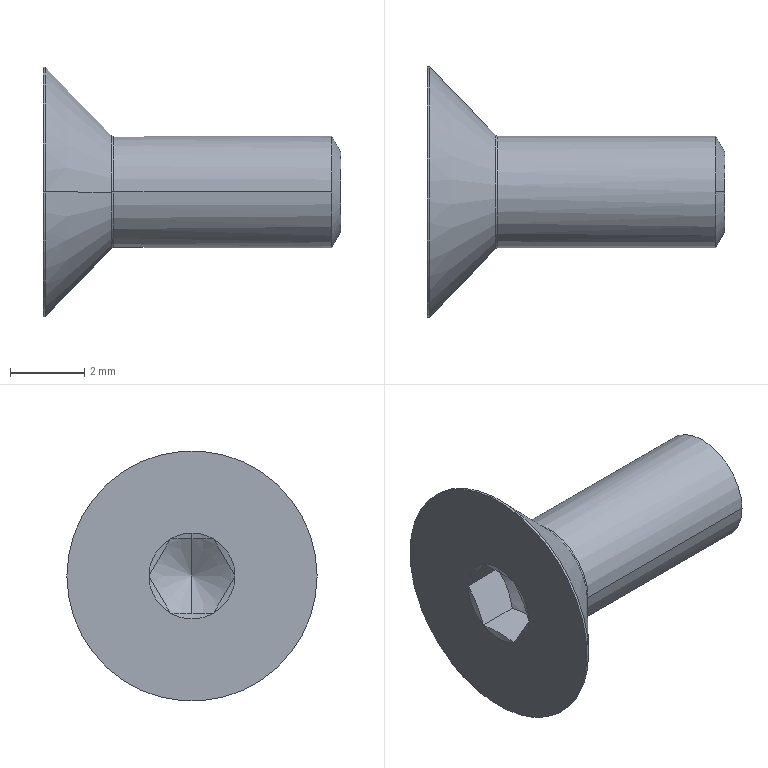Part | SolidWorks | features RevCut 2, Revolution 2, Cut 1, LPattern 1, RefAxis 1 | 1 solid | 27 faces | box 8 x 6.72 x 6.72 mm | volume 75.425 mm3 | cone 13 | plane 8 | cylinder 4 | torus 2 | commonest cylinder face diameters 3 x2 6.72 x2
STEP:
#1=CARTESIAN_POINT('',(0.,0.,1.067));
#2=VERTEX_POINT('',#1);
#3=CARTESIAN_POINT('',(0.,0.,-1.067));
#4=VERTEX_POINT('',#3);
#5=CARTESIAN_POINT('',(0.,0.,0.));
#6=DIRECTION('',(-1.,0.,0.));
#7=DIRECTION('',(0.,0.,1.));
#8=AXIS2_PLACEMENT_3D('',#5,#6,#7);
#9=CIRCLE('',#8,1.067);
#10=EDGE_CURVE('',#2,#4,#9,.T.);
#11=ORIENTED_EDGE('',*,*,#10,.T.);
#12=CARTESIAN_POINT('',(-0.25,0.,-1.5));
#13=VERTEX_POINT('',#12);
#14=CARTESIAN_POINT('',(-0.25,0.,-1.5));
#15=DIRECTION('',(-0.5,0.,-0.866));
#16=VECTOR('',#15,1000.);
#17=LINE('',#14,#16);
#18=EDGE_CURVE('',#4,#13,#17,.T.);
#19=ORIENTED_EDGE('',*,*,#18,.T.);
#20=CARTESIAN_POINT('',(-0.25,1.5,0.));
#21=VERTEX_POINT('',#20);
#22=CARTESIAN_POINT('',(-0.25,0.,0.));
#23=DIRECTION('',(-1.,0.,0.));
#24=DIRECTION('',(0.,0.,1.));
#25=AXIS2_PLACEMENT_3D('',#22,#23,#24);
#26=CIRCLE('',#25,1.5);
#27=EDGE_CURVE('',#21,#13,#26,.T.);
#28=ORIENTED_EDGE('',*,*,#27,.F.);
#29=CARTESIAN_POINT('',(-0.25,0.,1.5));
#30=VERTEX_POINT('',#29);
#31=CARTESIAN_POINT('',(-0.25,0.,0.));
#32=DIRECTION('',(-1.,0.,0.));
#33=DIRECTION('',(0.,0.,1.));
#34=AXIS2_PLACEMENT_3D('',#31,#32,#33);
#35=CIRCLE('',#34,1.5);
#36=EDGE_CURVE('',#30,#21,#35,.T.);
#37=ORIENTED_EDGE('',*,*,#36,.F.);
#38=CARTESIAN_POINT('',(-0.25,0.,1.5));
#39=DIRECTION('',(-0.5,0.,0.866));
#40=VECTOR('',#39,1000.);
#41=LINE('',#38,#40);
#42=EDGE_CURVE('',#2,#30,#41,.T.);
#43=ORIENTED_EDGE('',*,*,#42,.F.);
#44=EDGE_LOOP('',(#11,#19,#28,#37,#43));
#45=FACE_OUTER_BOUND('',#44,.T.);
#46=CARTESIAN_POINT('',(-0.25,0.,0.));
#47=DIRECTION('',(-1.,0.,0.));
#48=DIRECTION('',(0.,0.,1.));
#49=AXIS2_PLACEMENT_3D('',#46,#47,#48);
#50=CONICAL_SURFACE('',#49,1.5,1.047);
#51=ADVANCED_FACE('',(#45),#50,.T.);
#52=CARTESIAN_POINT('',(-6.233,0.,0.));
#53=VERTEX_POINT('',#52);
#54=CARTESIAN_POINT('',(-6.811,0.,1.));
#55=VERTEX_POINT('',#54);
#56=CARTESIAN_POINT('',(-6.9,0.,1.155));
#57=DIRECTION('',(-0.5,0.,0.866));
#58=VECTOR('',#57,1000.);
#59=LINE('',#56,#58);
#60=EDGE_CURVE('',#53,#55,#59,.T.);
#61=ORIENTED_EDGE('',*,*,#60,.F.);
#62=CARTESIAN_POINT('',(-6.811,0.,-1.));
#63=VERTEX_POINT('',#62);
#64=CARTESIAN_POINT('',(-6.9,0.,-1.155));
#65=DIRECTION('',(-0.5,0.,-0.866));
#66=VECTOR('',#65,1000.);
#67=LINE('',#64,#66);
#68=EDGE_CURVE('',#53,#63,#67,.T.);
#69=ORIENTED_EDGE('',*,*,#68,.T.);
#70=CARTESIAN_POINT('',(-6.9,-0.5774,-1.));
#71=VERTEX_POINT('',#70);
#72=CARTESIAN_POINT('',(-6.811,0.,-1.));
#73=CARTESIAN_POINT('',(-6.811,-0.1949,-1.));
#74=CARTESIAN_POINT('',(-6.846,-0.3898,-1.));
#75=CARTESIAN_POINT('',(-6.9,-0.5774,-1.));
#76=B_SPLINE_CURVE_WITH_KNOTS('',3,(#72,#73,#74,#75),.UNSPECIFIED.,.F.,.F.,(4,4),(0.003677,0.004261),.UNSPECIFIED.);
#77=EDGE_CURVE('',#63,#71,#76,.T.);
#78=ORIENTED_EDGE('',*,*,#77,.T.);
#79=CARTESIAN_POINT('',(-6.9,-1.155,0.));
#80=VERTEX_POINT('',#79);
#81=CARTESIAN_POINT('',(-6.9,-0.5774,-1.));
#82=CARTESIAN_POINT('',(-6.846,-0.6716,-0.8367));
#83=CARTESIAN_POINT('',(-6.811,-0.7673,-0.671));
#84=CARTESIAN_POINT('',(-6.811,-0.9636,-0.3309));
#85=CARTESIAN_POINT('',(-6.846,-1.06,-0.1635));
#86=CARTESIAN_POINT('',(-6.9,-1.155,0.));
#87=B_SPLINE_CURVE_WITH_KNOTS('',3,(#81,#82,#83,#84,#85,#86),.UNSPECIFIED.,.F.,.F.,(4,2,4),(0.000000238,0.0005833,0.001166),.UNSPECIFIED.);
#88=EDGE_CURVE('',#71,#80,#87,.T.);
#89=ORIENTED_EDGE('',*,*,#88,.T.);
#90=CARTESIAN_POINT('',(-6.9,-0.5774,1.));
#91=VERTEX_POINT('',#90);
#92=CARTESIAN_POINT('',(-6.9,-1.155,0.));
#93=CARTESIAN_POINT('',(-6.846,-1.06,0.1633));
#94=CARTESIAN_POINT('',(-6.811,-0.9647,0.329));
#95=CARTESIAN_POINT('',(-6.811,-0.7684,0.6691));
#96=CARTESIAN_POINT('',(-6.846,-0.6717,0.8365));
#97=CARTESIAN_POINT('',(-6.9,-0.5774,1.));
#98=B_SPLINE_CURVE_WITH_KNOTS('',3,(#92,#93,#94,#95,#96,#97),.UNSPECIFIED.,.F.,.F.,(4,2,4),(0.000000238,0.0005833,0.001166),.UNSPECIFIED.);
#99=EDGE_CURVE('',#80,#91,#98,.T.);
#100=ORIENTED_EDGE('',*,*,#99,.T.);
#101=CARTESIAN_POINT('',(-6.9,-0.5774,1.));
#102=CARTESIAN_POINT('',(-6.846,-0.3898,1.));
#103=CARTESIAN_POINT('',(-6.811,-0.1949,1.));
#104=CARTESIAN_POINT('',(-6.811,0.,1.));
#105=B_SPLINE_CURVE_WITH_KNOTS('',3,(#101,#102,#103,#104),.UNSPECIFIED.,.F.,.F.,(4,4),(0.00099,0.001574),.UNSPECIFIED.);
#106=EDGE_CURVE('',#91,#55,#105,.T.);
#107=ORIENTED_EDGE('',*,*,#106,.T.);
#108=EDGE_LOOP('',(#61,#69,#78,#89,#100,#107));
#109=FACE_OUTER_BOUND('',#108,.T.);
#110=CARTESIAN_POINT('',(-6.9,0.,0.));
#111=DIRECTION('',(-1.,0.,0.));
#112=DIRECTION('',(0.,0.,1.));
#113=AXIS2_PLACEMENT_3D('',#110,#111,#112);
#114=CONICAL_SURFACE('',#113,1.155,1.047);
#115=ADVANCED_FACE('',(#109),#114,.F.);
#116=CARTESIAN_POINT('',(-8.,0.5774,1.));
#117=VERTEX_POINT('',#116);
#118=CARTESIAN_POINT('',(-7.956,0.,1.));
#119=VERTEX_POINT('',#118);
#120=CARTESIAN_POINT('',(-8.,0.5774,1.));
#121=CARTESIAN_POINT('',(-7.973,0.3853,1.));
#122=CARTESIAN_POINT('',(-7.956,0.193,1.));
#123=CARTESIAN_POINT('',(-7.956,0.,1.));
#124=B_SPLINE_CURVE_WITH_KNOTS('',3,(#120,#121,#122,#123),.UNSPECIFIED.,.F.,.F.,(4,4),(0.002431,0.003013),.UNSPECIFIED.);
#125=EDGE_CURVE('',#117,#119,#124,.T.);
#126=ORIENTED_EDGE('',*,*,#125,.T.);
#127=CARTESIAN_POINT('',(-8.,0.,1.155));
#128=VERTEX_POINT('',#127);
#129=CARTESIAN_POINT('',(-7.67,0.,0.));
#130=DIRECTION('',(-0.2748,0.,0.9615));
#131=VECTOR('',#130,1000.);
#132=LINE('',#129,#131);
#133=EDGE_CURVE('',#119,#128,#132,.T.);
#134=ORIENTED_EDGE('',*,*,#133,.T.);
#135=CARTESIAN_POINT('',(-8.,0.,0.));
#136=DIRECTION('',(1.,0.,0.));
#137=DIRECTION('',(0.,-1.,0.));
#138=AXIS2_PLACEMENT_3D('',#135,#136,#137);
#139=CIRCLE('',#138,1.155);
#140=EDGE_CURVE('',#117,#128,#139,.T.);
#141=ORIENTED_EDGE('',*,*,#140,.F.);
#142=EDGE_LOOP('',(#126,#134,#141));
#143=FACE_OUTER_BOUND('',#142,.T.);
#144=CARTESIAN_POINT('',(-1007.67,0.,0.));
#145=DIRECTION('',(-1.,0.,0.));
#146=DIRECTION('',(0.,0.,1.));
#147=AXIS2_PLACEMENT_3D('',#144,#145,#146);
#148=CONICAL_SURFACE('',#147,3499.093,1.292);
#149=ADVANCED_FACE('',(#143),#148,.F.);
#150=CARTESIAN_POINT('',(-6.098,-1.5,0.));
#151=VERTEX_POINT('',#150);
#152=CARTESIAN_POINT('',(-6.098,1.5,0.));
#153=VERTEX_POINT('',#152);
#154=CARTESIAN_POINT('',(-6.098,0.,0.));
#155=DIRECTION('',(1.,0.,0.));
#156=DIRECTION('',(0.,1.,0.));
#157=AXIS2_PLACEMENT_3D('',#154,#155,#156);
#158=CIRCLE('',#157,1.5);
#159=EDGE_CURVE('',#151,#153,#158,.T.);
#160=ORIENTED_EDGE('',*,*,#159,.F.);
#161=CARTESIAN_POINT('',(-6.169,-1.531,0.));
#162=VERTEX_POINT('',#161);
#163=CARTESIAN_POINT('',(-6.098,-1.6,0.));
#164=DIRECTION('',(0.,0.,1.));
#165=DIRECTION('',(0.,-1.,0.));
#166=AXIS2_PLACEMENT_3D('',#163,#164,#165);
#167=CIRCLE('',#166,0.1);
#168=EDGE_CURVE('',#151,#162,#167,.T.);
#169=ORIENTED_EDGE('',*,*,#168,.T.);
#170=CARTESIAN_POINT('',(-6.169,1.531,0.));
#171=VERTEX_POINT('',#170);
#172=CARTESIAN_POINT('',(-6.169,0.,0.));
#173=DIRECTION('',(1.,0.,0.));
#174=DIRECTION('',(0.,1.,0.));
#175=AXIS2_PLACEMENT_3D('',#172,#173,#174);
#176=CIRCLE('',#175,1.531);
#177=EDGE_CURVE('',#162,#171,#176,.T.);
#178=ORIENTED_EDGE('',*,*,#177,.T.);
#179=CARTESIAN_POINT('',(-6.098,1.6,0.));
#180=DIRECTION('',(0.,0.,-1.));
#181=DIRECTION('',(-1.,0.,0.));
#182=AXIS2_PLACEMENT_3D('',#179,#180,#181);
#183=CIRCLE('',#182,0.1);
#184=EDGE_CURVE('',#153,#171,#183,.T.);
#185=ORIENTED_EDGE('',*,*,#184,.F.);
#186=EDGE_LOOP('',(#160,#169,#178,#185));
#187=FACE_OUTER_BOUND('',#186,.T.);
#188=CARTESIAN_POINT('',(-6.098,0.,0.));
#189=DIRECTION('',(1.,0.,0.));
#190=DIRECTION('',(0.,1.,0.));
#191=AXIS2_PLACEMENT_3D('',#188,#189,#190);
#192=TOROIDAL_SURFACE('',#191,1.6,0.1);
#193=ADVANCED_FACE('',(#187),#192,.F.);
#194=CARTESIAN_POINT('',(-6.169,0.,0.));
#195=DIRECTION('',(1.,0.,0.));
#196=DIRECTION('',(0.,1.,0.));
#197=AXIS2_PLACEMENT_3D('',#194,#195,#196);
#198=CIRCLE('',#197,1.531);
#199=EDGE_CURVE('',#171,#162,#198,.T.);
#200=ORIENTED_EDGE('',*,*,#199,.F.);
#201=CARTESIAN_POINT('',(-7.936,3.36,0.));
#202=VERTEX_POINT('',#201);
#203=CARTESIAN_POINT('',(-6.169,1.531,0.));
#204=DIRECTION('',(-0.6947,0.7193,0.));
#205=VECTOR('',#204,1000.);
#206=LINE('',#203,#205);
#207=EDGE_CURVE('',#171,#202,#206,.T.);
#208=ORIENTED_EDGE('',*,*,#207,.T.);
#209=CARTESIAN_POINT('',(-7.936,-3.36,0.));
#210=VERTEX_POINT('',#209);
#211=CARTESIAN_POINT('',(-7.936,0.,0.));
#212=DIRECTION('',(1.,0.,0.));
#213=DIRECTION('',(0.,1.,0.));
#214=AXIS2_PLACEMENT_3D('',#211,#212,#213);
#215=CIRCLE('',#214,3.36);
#216=EDGE_CURVE('',#202,#210,#215,.T.);
#217=ORIENTED_EDGE('',*,*,#216,.T.);
#218=CARTESIAN_POINT('',(-6.169,-1.531,0.));
#219=DIRECTION('',(-0.6947,-0.7193,0.));
#220=VECTOR('',#219,1000.);
#221=LINE('',#218,#220);
#222=EDGE_CURVE('',#162,#210,#221,.T.);
#223=ORIENTED_EDGE('',*,*,#222,.F.);
#224=EDGE_LOOP('',(#200,#208,#217,#223));
#225=FACE_OUTER_BOUND('',#224,.T.);
#226=CARTESIAN_POINT('',(-6.169,0.,0.));
#227=DIRECTION('',(-1.,0.,0.));
#228=DIRECTION('',(0.,-1.,0.));
#229=AXIS2_PLACEMENT_3D('',#226,#227,#228);
#230=CONICAL_SURFACE('',#229,1.531,0.8029);
#231=ADVANCED_FACE('',(#225),#230,.T.);
#232=CARTESIAN_POINT('',(-8.,3.36,0.));
#233=VERTEX_POINT('',#232);
#234=CARTESIAN_POINT('',(-8.,-3.36,0.));
#235=VERTEX_POINT('',#234);
#236=CARTESIAN_POINT('',(-8.,0.,0.));
#237=DIRECTION('',(1.,0.,0.));
#238=DIRECTION('',(0.,1.,0.));
#239=AXIS2_PLACEMENT_3D('',#236,#237,#238);
#240=CIRCLE('',#239,3.36);
#241=EDGE_CURVE('',#233,#235,#240,.T.);
#242=ORIENTED_EDGE('',*,*,#241,.T.);
#243=CARTESIAN_POINT('',(0.,-3.36,0.));
#244=DIRECTION('',(1.,0.,0.));
#245=VECTOR('',#244,1000.);
#246=LINE('',#243,#245);
#247=EDGE_CURVE('',#235,#210,#246,.T.);
#248=ORIENTED_EDGE('',*,*,#247,.T.);
#249=ORIENTED_EDGE('',*,*,#216,.F.);
#250=CARTESIAN_POINT('',(0.,3.36,0.));
#251=DIRECTION('',(1.,0.,0.));
#252=VECTOR('',#251,1000.);
#253=LINE('',#250,#252);
#254=EDGE_CURVE('',#233,#202,#253,.T.);
#255=ORIENTED_EDGE('',*,*,#254,.F.);
#256=EDGE_LOOP('',(#242,#248,#249,#255));
#257=FACE_OUTER_BOUND('',#256,.T.);
#258=CARTESIAN_POINT('',(0.,0.,0.));
#259=DIRECTION('',(1.,0.,0.));
#260=DIRECTION('',(0.,1.,0.));
#261=AXIS2_PLACEMENT_3D('',#258,#259,#260);
#262=CYLINDRICAL_SURFACE('',#261,3.36);
#263=ADVANCED_FACE('',(#257),#262,.T.);
#264=CARTESIAN_POINT('',(-6.098,0.,0.));
#265=DIRECTION('',(1.,0.,0.));
#266=DIRECTION('',(0.,1.,0.));
#267=AXIS2_PLACEMENT_3D('',#264,#265,#266);
#268=CIRCLE('',#267,1.5);
#269=EDGE_CURVE('',#153,#151,#268,.T.);
#270=ORIENTED_EDGE('',*,*,#269,.T.);
#271=CARTESIAN_POINT('',(-0.25,-1.5,0.));
#272=VERTEX_POINT('',#271);
#273=CARTESIAN_POINT('',(0.,-1.5,0.));
#274=DIRECTION('',(1.,0.,0.));
#275=VECTOR('',#274,1000.);
#276=LINE('',#273,#275);
#277=EDGE_CURVE('',#151,#272,#276,.T.);
#278=ORIENTED_EDGE('',*,*,#277,.T.);
#279=CARTESIAN_POINT('',(-0.25,0.,0.));
#280=DIRECTION('',(-1.,0.,0.));
#281=DIRECTION('',(0.,0.,1.));
#282=AXIS2_PLACEMENT_3D('',#279,#280,#281);
#283=CIRCLE('',#282,1.5);
#284=EDGE_CURVE('',#272,#30,#283,.T.);
#285=ORIENTED_EDGE('',*,*,#284,.T.);
#286=ORIENTED_EDGE('',*,*,#36,.T.);
#287=CARTESIAN_POINT('',(0.,1.5,0.));
#288=DIRECTION('',(1.,0.,0.));
#289=VECTOR('',#288,1000.);
#290=LINE('',#287,#289);
#291=EDGE_CURVE('',#153,#21,#290,.T.);
#292=ORIENTED_EDGE('',*,*,#291,.F.);
#293=EDGE_LOOP('',(#270,#278,#285,#286,#292));
#294=FACE_OUTER_BOUND('',#293,.T.);
#295=CARTESIAN_POINT('',(0.,0.,0.));
#296=DIRECTION('',(1.,0.,0.));
#297=DIRECTION('',(0.,1.,0.));
#298=AXIS2_PLACEMENT_3D('',#295,#296,#297);
#299=CYLINDRICAL_SURFACE('',#298,1.5);
#300=ADVANCED_FACE('',(#294),#299,.T.);
#301=ORIENTED_EDGE('',*,*,#277,.F.);
#302=ORIENTED_EDGE('',*,*,#159,.T.);
#303=ORIENTED_EDGE('',*,*,#291,.T.);
#304=ORIENTED_EDGE('',*,*,#27,.T.);
#305=CARTESIAN_POINT('',(-0.25,0.,0.));
#306=DIRECTION('',(-1.,0.,0.));
#307=DIRECTION('',(0.,0.,1.));
#308=AXIS2_PLACEMENT_3D('',#305,#306,#307);
#309=CIRCLE('',#308,1.5);
#310=EDGE_CURVE('',#13,#272,#309,.T.);
#311=ORIENTED_EDGE('',*,*,#310,.T.);
#312=EDGE_LOOP('',(#301,#302,#303,#304,#311));
#313=FACE_OUTER_BOUND('',#312,.T.);
#314=CARTESIAN_POINT('',(0.,0.,0.));
#315=DIRECTION('',(1.,0.,0.));
#316=DIRECTION('',(0.,1.,0.));
#317=AXIS2_PLACEMENT_3D('',#314,#315,#316);
#318=CYLINDRICAL_SURFACE('',#317,1.5);
#319=ADVANCED_FACE('',(#313),#318,.T.);
#320=ORIENTED_EDGE('',*,*,#241,.F.);
#321=CARTESIAN_POINT('',(-8.,0.,0.));
#322=DIRECTION('',(1.,0.,0.));
#323=DIRECTION('',(0.,1.,0.));
#324=AXIS2_PLACEMENT_3D('',#321,#322,#323);
#325=CIRCLE('',#324,3.36);
#326=EDGE_CURVE('',#235,#233,#325,.T.);
#327=ORIENTED_EDGE('',*,*,#326,.F.);
#328=EDGE_LOOP('',(#320,#327));
#329=FACE_OUTER_BOUND('',#328,.T.);
#330=CARTESIAN_POINT('',(-8.,-0.5774,1.));
#331=VERTEX_POINT('',#330);
#332=CARTESIAN_POINT('',(-8.,-1.155,0.));
#333=VERTEX_POINT('',#332);
#334=CARTESIAN_POINT('',(-8.,0.,0.));
#335=DIRECTION('',(1.,0.,0.));
#336=DIRECTION('',(0.,-1.,0.));
#337=AXIS2_PLACEMENT_3D('',#334,#335,#336);
#338=CIRCLE('',#337,1.155);
#339=EDGE_CURVE('',#331,#333,#338,.T.);
#340=ORIENTED_EDGE('',*,*,#339,.T.);
#341=CARTESIAN_POINT('',(-8.,-0.5774,-1.));
#342=VERTEX_POINT('',#341);
#343=CARTESIAN_POINT('',(-8.,0.,0.));
#344=DIRECTION('',(1.,0.,0.));
#345=DIRECTION('',(0.,-1.,0.));
#346=AXIS2_PLACEMENT_3D('',#343,#344,#345);
#347=CIRCLE('',#346,1.155);
#348=EDGE_CURVE('',#333,#342,#347,.T.);
#349=ORIENTED_EDGE('',*,*,#348,.T.);
#350=CARTESIAN_POINT('',(-8.,0.5774,-1.));
#351=VERTEX_POINT('',#350);
#352=CARTESIAN_POINT('',(-8.,0.,0.));
#353=DIRECTION('',(1.,0.,0.));
#354=DIRECTION('',(0.,-1.,0.));
#355=AXIS2_PLACEMENT_3D('',#352,#353,#354);
#356=CIRCLE('',#355,1.155);
#357=EDGE_CURVE('',#342,#351,#356,.T.);
#358=ORIENTED_EDGE('',*,*,#357,.T.);
#359=CARTESIAN_POINT('',(-8.,1.155,0.));
#360=VERTEX_POINT('',#359);
#361=CARTESIAN_POINT('',(-8.,0.,0.));
#362=DIRECTION('',(1.,0.,0.));
#363=DIRECTION('',(0.,-1.,0.));
#364=AXIS2_PLACEMENT_3D('',#361,#362,#363);
#365=CIRCLE('',#364,1.155);
#366=EDGE_CURVE('',#351,#360,#365,.T.);
#367=ORIENTED_EDGE('',*,*,#366,.T.);
#368=CARTESIAN_POINT('',(-8.,0.,0.));
#369=DIRECTION('',(-1.,0.,0.));
#370=DIRECTION('',(0.,0.,1.));
#371=AXIS2_PLACEMENT_3D('',#368,#369,#370);
#372=CIRCLE('',#371,1.155);
#373=EDGE_CURVE('',#117,#360,#372,.T.);
#374=ORIENTED_EDGE('',*,*,#373,.F.);
#375=ORIENTED_EDGE('',*,*,#140,.T.);
#376=CARTESIAN_POINT('',(-8.,0.,0.));
#377=DIRECTION('',(1.,0.,0.));
#378=DIRECTION('',(0.,-1.,0.));
#379=AXIS2_PLACEMENT_3D('',#376,#377,#378);
#380=CIRCLE('',#379,1.155);
#381=EDGE_CURVE('',#128,#331,#380,.T.);
#382=ORIENTED_EDGE('',*,*,#381,.T.);
#383=EDGE_LOOP('',(#340,#349,#358,#367,#374,#375,#382));
#384=FACE_BOUND('',#383,.T.);
#385=CARTESIAN_POINT('',(-8.,3.36,0.));
#386=DIRECTION('',(-1.,0.,0.));
#387=DIRECTION('',(0.,-1.,0.));
#388=AXIS2_PLACEMENT_3D('',#385,#386,#387);
#389=PLANE('',#388);
#390=ADVANCED_FACE('',(#329,#384),#389,.T.);
#391=ORIENTED_EDGE('',*,*,#247,.F.);
#392=ORIENTED_EDGE('',*,*,#326,.T.);
#393=ORIENTED_EDGE('',*,*,#254,.T.);
#394=CARTESIAN_POINT('',(-7.936,0.,0.));
#395=DIRECTION('',(1.,0.,0.));
#396=DIRECTION('',(0.,1.,0.));
#397=AXIS2_PLACEMENT_3D('',#394,#395,#396);
#398=CIRCLE('',#397,3.36);
#399=EDGE_CURVE('',#210,#202,#398,.T.);
#400=ORIENTED_EDGE('',*,*,#399,.F.);
#401=EDGE_LOOP('',(#391,#392,#393,#400));
#402=FACE_OUTER_BOUND('',#401,.T.);
#403=CARTESIAN_POINT('',(0.,0.,0.));
#404=DIRECTION('',(1.,0.,0.));
#405=DIRECTION('',(0.,1.,0.));
#406=AXIS2_PLACEMENT_3D('',#403,#404,#405);
#407=CYLINDRICAL_SURFACE('',#406,3.36);
#408=ADVANCED_FACE('',(#402),#407,.T.);
#409=ORIENTED_EDGE('',*,*,#207,.F.);
#410=ORIENTED_EDGE('',*,*,#177,.F.);
#411=ORIENTED_EDGE('',*,*,#222,.T.);
#412=ORIENTED_EDGE('',*,*,#399,.T.);
#413=EDGE_LOOP('',(#409,#410,#411,#412));
#414=FACE_OUTER_BOUND('',#413,.T.);
#415=CARTESIAN_POINT('',(-6.169,0.,0.));
#416=DIRECTION('',(-1.,0.,0.));
#417=DIRECTION('',(0.,-1.,0.));
#418=AXIS2_PLACEMENT_3D('',#415,#416,#417);
#419=CONICAL_SURFACE('',#418,1.531,0.8029);
#420=ADVANCED_FACE('',(#414),#419,.T.);
#421=ORIENTED_EDGE('',*,*,#168,.F.);
#422=ORIENTED_EDGE('',*,*,#269,.F.);
#423=ORIENTED_EDGE('',*,*,#184,.T.);
#424=ORIENTED_EDGE('',*,*,#199,.T.);
#425=EDGE_LOOP('',(#421,#422,#423,#424));
#426=FACE_OUTER_BOUND('',#425,.T.);
#427=CARTESIAN_POINT('',(-6.098,0.,0.));
#428=DIRECTION('',(1.,0.,0.));
#429=DIRECTION('',(0.,1.,0.));
#430=AXIS2_PLACEMENT_3D('',#427,#428,#429);
#431=TOROIDAL_SURFACE('',#430,1.6,0.1);
#432=ADVANCED_FACE('',(#426),#431,.F.);
#433=CARTESIAN_POINT('',(-8.,-0.5774,1.));
#434=CARTESIAN_POINT('',(-7.972,-0.6736,0.8333));
#435=CARTESIAN_POINT('',(-7.939,-0.866,0.5));
#436=CARTESIAN_POINT('',(-7.972,-1.058,0.1667));
#437=CARTESIAN_POINT('',(-8.,-1.155,0.));
#438=B_SPLINE_CURVE_WITH_KNOTS('',3,(#433,#434,#435,#436,#437),.UNSPECIFIED.,.F.,.F.,(4,1,4),(0.000000231,0.0005776,0.001155),.UNSPECIFIED.);
#439=EDGE_CURVE('',#331,#333,#438,.T.);
#440=ORIENTED_EDGE('',*,*,#439,.T.);
#441=ORIENTED_EDGE('',*,*,#339,.F.);
#442=EDGE_LOOP('',(#440,#441));
#443=FACE_OUTER_BOUND('',#442,.T.);
#444=CARTESIAN_POINT('',(-1007.67,0.,0.));
#445=DIRECTION('',(-1.,0.,0.));
#446=DIRECTION('',(0.,0.,1.));
#447=AXIS2_PLACEMENT_3D('',#444,#445,#446);
#448=CONICAL_SURFACE('',#447,3499.093,1.292);
#449=ADVANCED_FACE('',(#443),#448,.F.);
#450=ORIENTED_EDGE('',*,*,#133,.F.);
#451=CARTESIAN_POINT('',(-7.956,0.,1.));
#452=CARTESIAN_POINT('',(-7.956,-0.1921,1.));
#453=CARTESIAN_POINT('',(-7.973,-0.3856,1.));
#454=CARTESIAN_POINT('',(-8.,-0.5774,1.));
#455=B_SPLINE_CURVE_WITH_KNOTS('',3,(#451,#452,#453,#454),.UNSPECIFIED.,.F.,.F.,(4,4),(0.003013,0.003592),.UNSPECIFIED.);
#456=EDGE_CURVE('',#119,#331,#455,.T.);
#457=ORIENTED_EDGE('',*,*,#456,.T.);
#458=ORIENTED_EDGE('',*,*,#381,.F.);
#459=EDGE_LOOP('',(#450,#457,#458));
#460=FACE_OUTER_BOUND('',#459,.T.);
#461=CARTESIAN_POINT('',(-1007.67,0.,0.));
#462=DIRECTION('',(-1.,0.,0.));
#463=DIRECTION('',(0.,0.,1.));
#464=AXIS2_PLACEMENT_3D('',#461,#462,#463);
#465=CONICAL_SURFACE('',#464,3499.093,1.292);
#466=ADVANCED_FACE('',(#460),#465,.F.);
#467=CARTESIAN_POINT('',(-8.,1.155,0.));
#468=CARTESIAN_POINT('',(-7.972,1.058,0.1667));
#469=CARTESIAN_POINT('',(-7.939,0.866,0.5));
#470=CARTESIAN_POINT('',(-7.972,0.6736,0.8333));
#471=CARTESIAN_POINT('',(-8.,0.5774,1.));
#472=B_SPLINE_CURVE_WITH_KNOTS('',3,(#467,#468,#469,#470,#471),.UNSPECIFIED.,.F.,.F.,(4,1,4),(0.000000231,0.0005776,0.001155),.UNSPECIFIED.);
#473=EDGE_CURVE('',#360,#117,#472,.T.);
#474=ORIENTED_EDGE('',*,*,#473,.T.);
#475=ORIENTED_EDGE('',*,*,#373,.T.);
#476=EDGE_LOOP('',(#474,#475));
#477=FACE_OUTER_BOUND('',#476,.T.);
#478=CARTESIAN_POINT('',(-1007.67,0.,0.));
#479=DIRECTION('',(-1.,0.,0.));
#480=DIRECTION('',(0.,0.,1.));
#481=AXIS2_PLACEMENT_3D('',#478,#479,#480);
#482=CONICAL_SURFACE('',#481,3499.093,1.292);
#483=ADVANCED_FACE('',(#477),#482,.F.);
#484=CARTESIAN_POINT('',(-8.,0.5774,-1.));
#485=CARTESIAN_POINT('',(-7.972,0.6736,-0.8333));
#486=CARTESIAN_POINT('',(-7.939,0.866,-0.5));
#487=CARTESIAN_POINT('',(-7.972,1.058,-0.1667));
#488=CARTESIAN_POINT('',(-8.,1.155,0.));
#489=B_SPLINE_CURVE_WITH_KNOTS('',3,(#484,#485,#486,#487,#488),.UNSPECIFIED.,.F.,.F.,(4,1,4),(0.000000231,0.0005776,0.001155),.UNSPECIFIED.);
#490=EDGE_CURVE('',#351,#360,#489,.T.);
#491=ORIENTED_EDGE('',*,*,#490,.T.);
#492=ORIENTED_EDGE('',*,*,#366,.F.);
#493=EDGE_LOOP('',(#491,#492));
#494=FACE_OUTER_BOUND('',#493,.T.);
#495=CARTESIAN_POINT('',(-1007.67,0.,0.));
#496=DIRECTION('',(-1.,0.,0.));
#497=DIRECTION('',(0.,0.,1.));
#498=AXIS2_PLACEMENT_3D('',#495,#496,#497);
#499=CONICAL_SURFACE('',#498,3499.093,1.292);
#500=ADVANCED_FACE('',(#494),#499,.F.);
#501=CARTESIAN_POINT('',(-8.,-0.5774,-1.));
#502=CARTESIAN_POINT('',(-7.973,-0.3852,-1.));
#503=CARTESIAN_POINT('',(-7.956,-0.1913,-1.));
#504=CARTESIAN_POINT('',(-7.956,0.1938,-1.));
#505=CARTESIAN_POINT('',(-7.973,0.3858,-1.));
#506=CARTESIAN_POINT('',(-8.,0.5774,-1.));
#507=B_SPLINE_CURVE_WITH_KNOTS('',3,(#501,#502,#503,#504,#505,#506),.UNSPECIFIED.,.F.,.F.,(4,2,4),(0.0009462,0.001528,0.002109),.UNSPECIFIED.);
#508=EDGE_CURVE('',#342,#351,#507,.T.);
#509=ORIENTED_EDGE('',*,*,#508,.T.);
#510=ORIENTED_EDGE('',*,*,#357,.F.);
#511=EDGE_LOOP('',(#509,#510));
#512=FACE_OUTER_BOUND('',#511,.T.);
#513=CARTESIAN_POINT('',(-1007.67,0.,0.));
#514=DIRECTION('',(-1.,0.,0.));
#515=DIRECTION('',(0.,0.,1.));
#516=AXIS2_PLACEMENT_3D('',#513,#514,#515);
#517=CONICAL_SURFACE('',#516,3499.093,1.292);
#518=ADVANCED_FACE('',(#512),#517,.F.);
#519=CARTESIAN_POINT('',(-8.,-1.155,0.));
#520=CARTESIAN_POINT('',(-7.972,-1.058,-0.1667));
#521=CARTESIAN_POINT('',(-7.939,-0.866,-0.5));
#522=CARTESIAN_POINT('',(-7.972,-0.6736,-0.8333));
#523=CARTESIAN_POINT('',(-8.,-0.5774,-1.));
#524=B_SPLINE_CURVE_WITH_KNOTS('',3,(#519,#520,#521,#522,#523),.UNSPECIFIED.,.F.,.F.,(4,1,4),(0.000000231,0.0005776,0.001155),.UNSPECIFIED.);
#525=EDGE_CURVE('',#333,#342,#524,.T.);
#526=ORIENTED_EDGE('',*,*,#525,.T.);
#527=ORIENTED_EDGE('',*,*,#348,.F.);
#528=EDGE_LOOP('',(#526,#527));
#529=FACE_OUTER_BOUND('',#528,.T.);
#530=CARTESIAN_POINT('',(-1007.67,0.,0.));
#531=DIRECTION('',(-1.,0.,0.));
#532=DIRECTION('',(0.,0.,1.));
#533=AXIS2_PLACEMENT_3D('',#530,#531,#532);
#534=CONICAL_SURFACE('',#533,3499.093,1.292);
#535=ADVANCED_FACE('',(#529),#534,.F.);
#536=ORIENTED_EDGE('',*,*,#68,.F.);
#537=ORIENTED_EDGE('',*,*,#60,.T.);
#538=CARTESIAN_POINT('',(-6.9,0.5774,1.));
#539=VERTEX_POINT('',#538);
#540=CARTESIAN_POINT('',(-6.811,0.,1.));
#541=CARTESIAN_POINT('',(-6.811,0.09751,1.));
#542=CARTESIAN_POINT('',(-6.819,0.1963,1.));
#543=CARTESIAN_POINT('',(-6.851,0.3894,1.));
#544=CARTESIAN_POINT('',(-6.873,0.484,1.));
#545=CARTESIAN_POINT('',(-6.9,0.5774,1.));
#546=B_SPLINE_CURVE_WITH_KNOTS('',3,(#540,#541,#542,#543,#544,#545),.UNSPECIFIED.,.F.,.F.,(4,2,4),(0.001574,0.001866,0.002158),.UNSPECIFIED.);
#547=EDGE_CURVE('',#55,#539,#546,.T.);
#548=ORIENTED_EDGE('',*,*,#547,.T.);
#549=CARTESIAN_POINT('',(-6.9,1.155,0.));
#550=VERTEX_POINT('',#549);
#551=CARTESIAN_POINT('',(-6.9,0.5774,1.));
#552=CARTESIAN_POINT('',(-6.846,0.6716,0.8367));
#553=CARTESIAN_POINT('',(-6.811,0.7673,0.671));
#554=CARTESIAN_POINT('',(-6.811,0.9636,0.3309));
#555=CARTESIAN_POINT('',(-6.846,1.06,0.1635));
#556=CARTESIAN_POINT('',(-6.9,1.155,0.));
#557=B_SPLINE_CURVE_WITH_KNOTS('',3,(#551,#552,#553,#554,#555,#556),.UNSPECIFIED.,.F.,.F.,(4,2,4),(0.000000238,0.0005833,0.001166),.UNSPECIFIED.);
#558=EDGE_CURVE('',#539,#550,#557,.T.);
#559=ORIENTED_EDGE('',*,*,#558,.T.);
#560=CARTESIAN_POINT('',(-6.9,0.5774,-1.));
#561=VERTEX_POINT('',#560);
#562=CARTESIAN_POINT('',(-6.9,1.155,0.));
#563=CARTESIAN_POINT('',(-6.846,1.06,-0.1633));
#564=CARTESIAN_POINT('',(-6.811,0.9647,-0.329));
#565=CARTESIAN_POINT('',(-6.811,0.7684,-0.6691));
#566=CARTESIAN_POINT('',(-6.846,0.6717,-0.8365));
#567=CARTESIAN_POINT('',(-6.9,0.5774,-1.));
#568=B_SPLINE_CURVE_WITH_KNOTS('',3,(#562,#563,#564,#565,#566,#567),.UNSPECIFIED.,.F.,.F.,(4,2,4),(0.000000238,0.0005833,0.001166),.UNSPECIFIED.);
#569=EDGE_CURVE('',#550,#561,#568,.T.);
#570=ORIENTED_EDGE('',*,*,#569,.T.);
#571=CARTESIAN_POINT('',(-6.9,0.5774,-1.));
#572=CARTESIAN_POINT('',(-6.873,0.484,-1.));
#573=CARTESIAN_POINT('',(-6.851,0.3894,-1.));
#574=CARTESIAN_POINT('',(-6.819,0.1963,-1.));
#575=CARTESIAN_POINT('',(-6.811,0.09751,-1.));
#576=CARTESIAN_POINT('',(-6.811,0.,-1.));
#577=B_SPLINE_CURVE_WITH_KNOTS('',3,(#571,#572,#573,#574,#575,#576),.UNSPECIFIED.,.F.,.F.,(4,2,4),(0.003092,0.003385,0.003677),.UNSPECIFIED.);
#578=EDGE_CURVE('',#561,#63,#577,.T.);
#579=ORIENTED_EDGE('',*,*,#578,.T.);
#580=EDGE_LOOP('',(#536,#537,#548,#559,#570,#579));
#581=FACE_OUTER_BOUND('',#580,.T.);
#582=CARTESIAN_POINT('',(-6.9,0.,0.));
#583=DIRECTION('',(-1.,0.,0.));
#584=DIRECTION('',(0.,0.,1.));
#585=AXIS2_PLACEMENT_3D('',#582,#583,#584);
#586=CONICAL_SURFACE('',#585,1.155,1.047);
#587=ADVANCED_FACE('',(#581),#586,.F.);
#588=ORIENTED_EDGE('',*,*,#490,.F.);
#589=CARTESIAN_POINT('',(-6.04,0.5774,-1.));
#590=DIRECTION('',(-1.,0.,0.));
#591=VECTOR('',#590,1000.);
#592=LINE('',#589,#591);
#593=EDGE_CURVE('',#561,#351,#592,.T.);
#594=ORIENTED_EDGE('',*,*,#593,.F.);
#595=ORIENTED_EDGE('',*,*,#569,.F.);
#596=CARTESIAN_POINT('',(-6.04,1.155,0.));
#597=DIRECTION('',(-1.,0.,0.));
#598=VECTOR('',#597,1000.);
#599=LINE('',#596,#598);
#600=EDGE_CURVE('',#550,#360,#599,.T.);
#601=ORIENTED_EDGE('',*,*,#600,.T.);
#602=EDGE_LOOP('',(#588,#594,#595,#601));
#603=FACE_OUTER_BOUND('',#602,.T.);
#604=CARTESIAN_POINT('',(-6.04,1.155,0.));
#605=DIRECTION('',(0.,0.866,-0.5));
#606=DIRECTION('',(0.,0.5,0.866));
#607=AXIS2_PLACEMENT_3D('',#604,#605,#606);
#608=PLANE('',#607);
#609=ADVANCED_FACE('',(#603),#608,.F.);
#610=ORIENTED_EDGE('',*,*,#508,.F.);
#611=CARTESIAN_POINT('',(-6.04,-0.5774,-1.));
#612=DIRECTION('',(-1.,0.,0.));
#613=VECTOR('',#612,1000.);
#614=LINE('',#611,#613);
#615=EDGE_CURVE('',#71,#342,#614,.T.);
#616=ORIENTED_EDGE('',*,*,#615,.F.);
#617=ORIENTED_EDGE('',*,*,#77,.F.);
#618=ORIENTED_EDGE('',*,*,#578,.F.);
#619=ORIENTED_EDGE('',*,*,#593,.T.);
#620=EDGE_LOOP('',(#610,#616,#617,#618,#619));
#621=FACE_OUTER_BOUND('',#620,.T.);
#622=CARTESIAN_POINT('',(-6.04,0.5774,-1.));
#623=DIRECTION('',(0.,0.,-1.));
#624=DIRECTION('',(-1.,0.,0.));
#625=AXIS2_PLACEMENT_3D('',#622,#623,#624);
#626=PLANE('',#625);
#627=ADVANCED_FACE('',(#621),#626,.F.);
#628=ORIENTED_EDGE('',*,*,#525,.F.);
#629=CARTESIAN_POINT('',(-6.04,-1.155,0.));
#630=DIRECTION('',(-1.,0.,0.));
#631=VECTOR('',#630,1000.);
#632=LINE('',#629,#631);
#633=EDGE_CURVE('',#80,#333,#632,.T.);
#634=ORIENTED_EDGE('',*,*,#633,.F.);
#635=ORIENTED_EDGE('',*,*,#88,.F.);
#636=ORIENTED_EDGE('',*,*,#615,.T.);
#637=EDGE_LOOP('',(#628,#634,#635,#636));
#638=FACE_OUTER_BOUND('',#637,.T.);
#639=CARTESIAN_POINT('',(-6.04,-0.5774,-1.));
#640=DIRECTION('',(0.,-0.866,-0.5));
#641=DIRECTION('',(0.,0.5,-0.866));
#642=AXIS2_PLACEMENT_3D('',#639,#640,#641);
#643=PLANE('',#642);
#644=ADVANCED_FACE('',(#638),#643,.F.);
#645=ORIENTED_EDGE('',*,*,#439,.F.);
#646=CARTESIAN_POINT('',(-6.04,-0.5774,1.));
#647=DIRECTION('',(-1.,0.,0.));
#648=VECTOR('',#647,1000.);
#649=LINE('',#646,#648);
#650=EDGE_CURVE('',#91,#331,#649,.T.);
#651=ORIENTED_EDGE('',*,*,#650,.F.);
#652=ORIENTED_EDGE('',*,*,#99,.F.);
#653=ORIENTED_EDGE('',*,*,#633,.T.);
#654=EDGE_LOOP('',(#645,#651,#652,#653));
#655=FACE_OUTER_BOUND('',#654,.T.);
#656=CARTESIAN_POINT('',(-6.04,-1.155,0.));
#657=DIRECTION('',(0.,-0.866,0.5));
#658=DIRECTION('',(0.,-0.5,-0.866));
#659=AXIS2_PLACEMENT_3D('',#656,#657,#658);
#660=PLANE('',#659);
#661=ADVANCED_FACE('',(#655),#660,.F.);
#662=ORIENTED_EDGE('',*,*,#125,.F.);
#663=CARTESIAN_POINT('',(-6.04,0.5774,1.));
#664=DIRECTION('',(-1.,0.,0.));
#665=VECTOR('',#664,1000.);
#666=LINE('',#663,#665);
#667=EDGE_CURVE('',#539,#117,#666,.T.);
#668=ORIENTED_EDGE('',*,*,#667,.F.);
#669=ORIENTED_EDGE('',*,*,#547,.F.);
#670=ORIENTED_EDGE('',*,*,#106,.F.);
#671=ORIENTED_EDGE('',*,*,#650,.T.);
#672=ORIENTED_EDGE('',*,*,#456,.F.);
#673=EDGE_LOOP('',(#662,#668,#669,#670,#671,#672));
#674=FACE_OUTER_BOUND('',#673,.T.);
#675=CARTESIAN_POINT('',(-6.04,-0.5774,1.));
#676=DIRECTION('',(0.,0.,1.));
#677=DIRECTION('',(1.,0.,0.));
#678=AXIS2_PLACEMENT_3D('',#675,#676,#677);
#679=PLANE('',#678);
#680=ADVANCED_FACE('',(#674),#679,.F.);
#681=ORIENTED_EDGE('',*,*,#473,.F.);
#682=ORIENTED_EDGE('',*,*,#600,.F.);
#683=ORIENTED_EDGE('',*,*,#558,.F.);
#684=ORIENTED_EDGE('',*,*,#667,.T.);
#685=EDGE_LOOP('',(#681,#682,#683,#684));
#686=FACE_OUTER_BOUND('',#685,.T.);
#687=CARTESIAN_POINT('',(-6.04,0.5774,1.));
#688=DIRECTION('',(0.,0.866,0.5));
#689=DIRECTION('',(0.,-0.5,0.866));
#690=AXIS2_PLACEMENT_3D('',#687,#688,#689);
#691=PLANE('',#690);
#692=ADVANCED_FACE('',(#686),#691,.F.);
#693=ORIENTED_EDGE('',*,*,#18,.F.);
#694=CARTESIAN_POINT('',(0.,0.,0.));
#695=DIRECTION('',(-1.,0.,0.));
#696=DIRECTION('',(0.,0.,1.));
#697=AXIS2_PLACEMENT_3D('',#694,#695,#696);
#698=CIRCLE('',#697,1.067);
#699=EDGE_CURVE('',#4,#2,#698,.T.);
#700=ORIENTED_EDGE('',*,*,#699,.T.);
#701=ORIENTED_EDGE('',*,*,#42,.T.);
#702=ORIENTED_EDGE('',*,*,#284,.F.);
#703=ORIENTED_EDGE('',*,*,#310,.F.);
#704=EDGE_LOOP('',(#693,#700,#701,#702,#703));
#705=FACE_OUTER_BOUND('',#704,.T.);
#706=CARTESIAN_POINT('',(-0.25,0.,0.));
#707=DIRECTION('',(-1.,0.,0.));
#708=DIRECTION('',(0.,0.,1.));
#709=AXIS2_PLACEMENT_3D('',#706,#707,#708);
#710=CONICAL_SURFACE('',#709,1.5,1.047);
#711=ADVANCED_FACE('',(#705),#710,.T.);
#712=ORIENTED_EDGE('',*,*,#10,.F.);
#713=ORIENTED_EDGE('',*,*,#699,.F.);
#714=EDGE_LOOP('',(#712,#713));
#715=FACE_OUTER_BOUND('',#714,.T.);
#716=CARTESIAN_POINT('',(0.,0.,0.));
#717=DIRECTION('',(1.,0.,0.));
#718=DIRECTION('',(0.,1.,0.));
#719=AXIS2_PLACEMENT_3D('',#716,#717,#718);
#720=PLANE('',#719);
#721=ADVANCED_FACE('',(#715),#720,.T.);
#722=CLOSED_SHELL('',(#51,#115,#149,#193,#231,#263,#300,#319,#390,#408,#420,#432,#449,#466,#483,#500,#518,#535,#587,#609,#627,#644,#661,#680,#692,#711,#721));
#723=MANIFOLD_SOLID_BREP('',#722);
#724=CARTESIAN_POINT('',(0.,0.,0.));
#725=DIRECTION('',(0.,0.,1.));
#726=DIRECTION('',(1.,0.,0.));
#727=AXIS2_PLACEMENT_3D('',#724,#725,#726);
#728=(LENGTH_UNIT()NAMED_UNIT(*)SI_UNIT(.MILLI.,.METRE.));
#729=UNCERTAINTY_MEASURE_WITH_UNIT(LENGTH_MEASURE(0.00001),#728,'','');
#730=(NAMED_UNIT(*)PLANE_ANGLE_UNIT()SI_UNIT($,.RADIAN.));
#731=(NAMED_UNIT(*)SI_UNIT($,.STERADIAN.)SOLID_ANGLE_UNIT());
#732=(GEOMETRIC_REPRESENTATION_CONTEXT(3)GLOBAL_UNCERTAINTY_ASSIGNED_CONTEXT((#729))GLOBAL_UNIT_ASSIGNED_CONTEXT((#728,#730,#731))REPRESENTATION_CONTEXT('',''));
#733=ADVANCED_BREP_SHAPE_REPRESENTATION('',(#723,#727),#732);